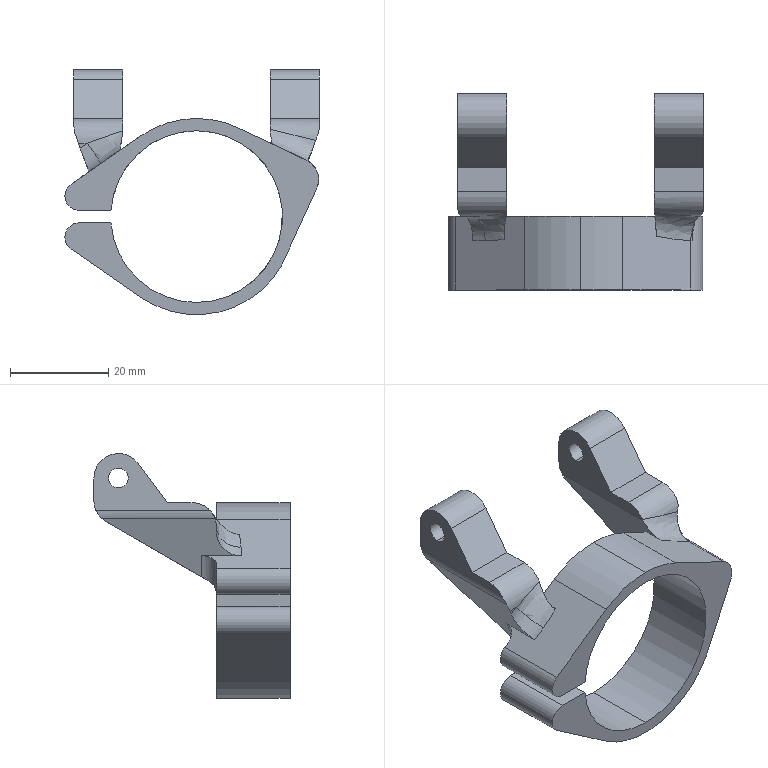Part | STEP file | Mounting Bracket v2 | 1 solid | 56 faces | box 51.858 x 40 x 50 mm | volume 13111 mm3 | plane 27 | cylinder 26 | spline 3 | commonest cylinder face diameters 10 x9 4 x4 6 x4 35 x3 40 x3 5.858 x2